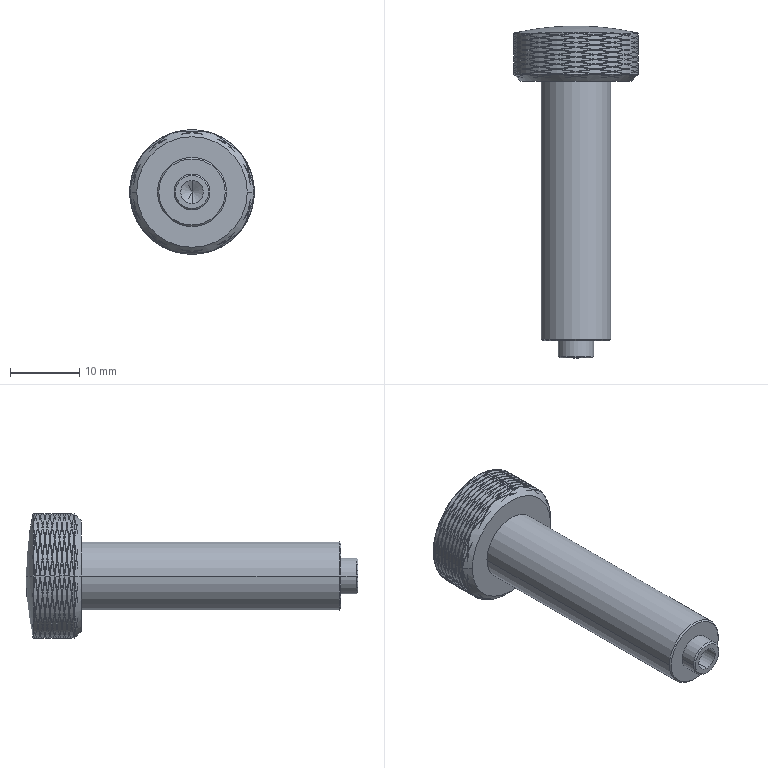Part | SolidWorks | features Helix 2, SweepCut 2, Chamfer 1, CirPattern 1, HoleWzd 1, Revolution 1 | 1 solid | 999 faces | box 18 x 48 x 18 mm | volume 4770 mm3 | spline 760 | cylinder 206 | cone 18 | plane 13 | sphere 2 | commonest cylinder face diameters 18 x200 3.3 x2 5.2 x2 10 x2